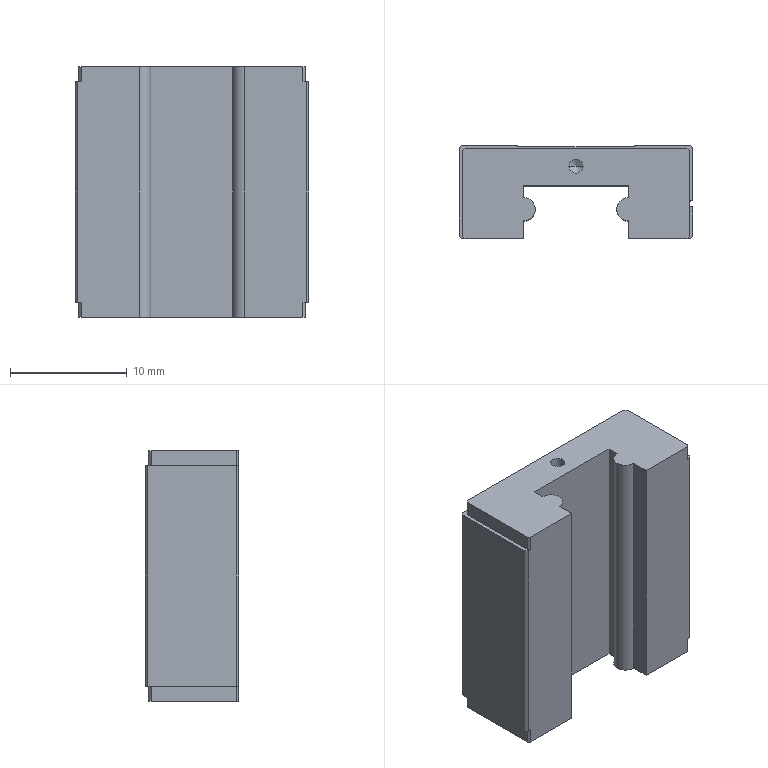Part | STEP file | MGN9S slider 1001 | 1 solid | 60 faces | box 20 x 8 x 21.5 mm | volume 2522 mm3 | plane 39 | cylinder 13 | cone 8 | commonest cylinder face diameters 1.2 x4 2.5 x4 2 x3 0.6 x2